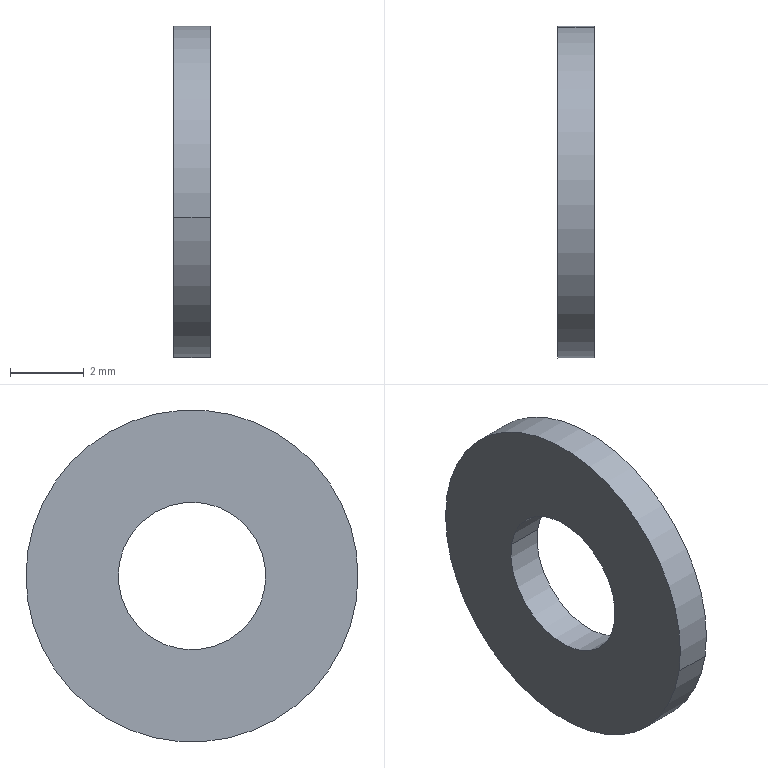Part | SolidWorks | features BaseBody 1 | 1 solid | 6 faces | box 1 x 9 x 9 mm | volume 51.051 mm3 | cylinder 4 | plane 2 | commonest cylinder face diameters 4 x2 9 x2
STEP:
#1=CARTESIAN_POINT('',(-440.148,436.692,-362.691));
#2=VERTEX_POINT('',#1);
#3=CARTESIAN_POINT('',(-440.148,432.739,-363.301));
#4=VERTEX_POINT('',#3);
#5=CARTESIAN_POINT('',(-440.148,434.715,-362.996));
#6=DIRECTION('',(1.,0.,0.));
#7=DIRECTION('',(0.,0.9883,0.1525));
#8=AXIS2_PLACEMENT_3D('',#5,#6,#7);
#9=CIRCLE('',#8,2.);
#10=EDGE_CURVE('',#2,#4,#9,.T.);
#11=ORIENTED_EDGE('',*,*,#10,.F.);
#12=CARTESIAN_POINT('',(-440.148,434.715,-362.996));
#13=DIRECTION('',(1.,0.,0.));
#14=DIRECTION('',(0.,-0.9883,-0.1525));
#15=AXIS2_PLACEMENT_3D('',#12,#13,#14);
#16=CIRCLE('',#15,2.);
#17=EDGE_CURVE('',#4,#2,#16,.T.);
#18=ORIENTED_EDGE('',*,*,#17,.F.);
#19=EDGE_LOOP('',(#11,#18));
#20=FACE_BOUND('',#19,.T.);
#21=CARTESIAN_POINT('',(-440.148,439.163,-362.31));
#22=VERTEX_POINT('',#21);
#23=CARTESIAN_POINT('',(-440.148,430.268,-363.683));
#24=VERTEX_POINT('',#23);
#25=CARTESIAN_POINT('',(-440.148,434.715,-362.996));
#26=DIRECTION('',(-1.,0.,0.));
#27=DIRECTION('',(0.,0.9883,0.1525));
#28=AXIS2_PLACEMENT_3D('',#25,#26,#27);
#29=CIRCLE('',#28,4.5);
#30=EDGE_CURVE('',#22,#24,#29,.T.);
#31=ORIENTED_EDGE('',*,*,#30,.F.);
#32=CARTESIAN_POINT('',(-440.148,434.715,-362.996));
#33=DIRECTION('',(-1.,0.,0.));
#34=DIRECTION('',(0.,-0.9883,-0.1525));
#35=AXIS2_PLACEMENT_3D('',#32,#33,#34);
#36=CIRCLE('',#35,4.5);
#37=EDGE_CURVE('',#24,#22,#36,.T.);
#38=ORIENTED_EDGE('',*,*,#37,.F.);
#39=EDGE_LOOP('',(#31,#38));
#40=FACE_OUTER_BOUND('',#39,.T.);
#41=CARTESIAN_POINT('',(-440.148,434.715,-362.996));
#42=DIRECTION('',(-1.,0.,0.));
#43=DIRECTION('',(0.,0.,1.));
#44=AXIS2_PLACEMENT_3D('',#41,#42,#43);
#45=PLANE('',#44);
#46=ADVANCED_FACE('',(#20,#40),#45,.F.);
#47=CARTESIAN_POINT('',(-441.148,439.163,-362.31));
#48=VERTEX_POINT('',#47);
#49=CARTESIAN_POINT('',(-440.148,439.163,-362.31));
#50=DIRECTION('',(-1.,0.,0.));
#51=VECTOR('',#50,1000.);
#52=LINE('',#49,#51);
#53=EDGE_CURVE('',#22,#48,#52,.T.);
#54=ORIENTED_EDGE('',*,*,#53,.T.);
#55=CARTESIAN_POINT('',(-441.148,430.268,-363.683));
#56=VERTEX_POINT('',#55);
#57=CARTESIAN_POINT('',(-441.148,434.715,-362.996));
#58=DIRECTION('',(1.,0.,0.));
#59=DIRECTION('',(0.,0.9883,0.1525));
#60=AXIS2_PLACEMENT_3D('',#57,#58,#59);
#61=CIRCLE('',#60,4.5);
#62=EDGE_CURVE('',#48,#56,#61,.T.);
#63=ORIENTED_EDGE('',*,*,#62,.T.);
#64=CARTESIAN_POINT('',(-440.148,430.268,-363.683));
#65=DIRECTION('',(-1.,0.,0.));
#66=VECTOR('',#65,1000.);
#67=LINE('',#64,#66);
#68=EDGE_CURVE('',#24,#56,#67,.T.);
#69=ORIENTED_EDGE('',*,*,#68,.F.);
#70=ORIENTED_EDGE('',*,*,#37,.T.);
#71=EDGE_LOOP('',(#54,#63,#69,#70));
#72=FACE_OUTER_BOUND('',#71,.T.);
#73=CARTESIAN_POINT('',(-440.148,434.715,-362.996));
#74=DIRECTION('',(-1.,0.,0.));
#75=DIRECTION('',(0.,-0.9883,-0.1525));
#76=AXIS2_PLACEMENT_3D('',#73,#74,#75);
#77=CYLINDRICAL_SURFACE('',#76,4.5);
#78=ADVANCED_FACE('',(#72),#77,.T.);
#79=ORIENTED_EDGE('',*,*,#68,.T.);
#80=CARTESIAN_POINT('',(-441.148,434.715,-362.996));
#81=DIRECTION('',(1.,0.,0.));
#82=DIRECTION('',(0.,-0.9883,-0.1525));
#83=AXIS2_PLACEMENT_3D('',#80,#81,#82);
#84=CIRCLE('',#83,4.5);
#85=EDGE_CURVE('',#56,#48,#84,.T.);
#86=ORIENTED_EDGE('',*,*,#85,.T.);
#87=ORIENTED_EDGE('',*,*,#53,.F.);
#88=ORIENTED_EDGE('',*,*,#30,.T.);
#89=EDGE_LOOP('',(#79,#86,#87,#88));
#90=FACE_OUTER_BOUND('',#89,.T.);
#91=CARTESIAN_POINT('',(-440.148,434.715,-362.996));
#92=DIRECTION('',(-1.,0.,0.));
#93=DIRECTION('',(0.,-0.9883,-0.1525));
#94=AXIS2_PLACEMENT_3D('',#91,#92,#93);
#95=CYLINDRICAL_SURFACE('',#94,4.5);
#96=ADVANCED_FACE('',(#90),#95,.T.);
#97=CARTESIAN_POINT('',(-441.148,432.739,-363.301));
#98=VERTEX_POINT('',#97);
#99=CARTESIAN_POINT('',(-441.148,436.692,-362.691));
#100=VERTEX_POINT('',#99);
#101=CARTESIAN_POINT('',(-441.148,434.715,-362.996));
#102=DIRECTION('',(-1.,0.,0.));
#103=DIRECTION('',(0.,-0.9883,-0.1525));
#104=AXIS2_PLACEMENT_3D('',#101,#102,#103);
#105=CIRCLE('',#104,2.);
#106=EDGE_CURVE('',#98,#100,#105,.T.);
#107=ORIENTED_EDGE('',*,*,#106,.F.);
#108=CARTESIAN_POINT('',(-441.148,434.715,-362.996));
#109=DIRECTION('',(-1.,0.,0.));
#110=DIRECTION('',(0.,0.9883,0.1525));
#111=AXIS2_PLACEMENT_3D('',#108,#109,#110);
#112=CIRCLE('',#111,2.);
#113=EDGE_CURVE('',#100,#98,#112,.T.);
#114=ORIENTED_EDGE('',*,*,#113,.F.);
#115=EDGE_LOOP('',(#107,#114));
#116=FACE_BOUND('',#115,.T.);
#117=ORIENTED_EDGE('',*,*,#85,.F.);
#118=ORIENTED_EDGE('',*,*,#62,.F.);
#119=EDGE_LOOP('',(#117,#118));
#120=FACE_OUTER_BOUND('',#119,.T.);
#121=CARTESIAN_POINT('',(-441.148,434.715,-362.996));
#122=DIRECTION('',(-1.,0.,0.));
#123=DIRECTION('',(0.,0.,1.));
#124=AXIS2_PLACEMENT_3D('',#121,#122,#123);
#125=PLANE('',#124);
#126=ADVANCED_FACE('',(#116,#120),#125,.T.);
#127=CARTESIAN_POINT('',(-440.148,436.692,-362.691));
#128=DIRECTION('',(-1.,0.,0.));
#129=VECTOR('',#128,1000.);
#130=LINE('',#127,#129);
#131=EDGE_CURVE('',#2,#100,#130,.T.);
#132=ORIENTED_EDGE('',*,*,#131,.T.);
#133=ORIENTED_EDGE('',*,*,#113,.T.);
#134=CARTESIAN_POINT('',(-440.148,432.739,-363.301));
#135=DIRECTION('',(-1.,0.,0.));
#136=VECTOR('',#135,1000.);
#137=LINE('',#134,#136);
#138=EDGE_CURVE('',#4,#98,#137,.T.);
#139=ORIENTED_EDGE('',*,*,#138,.F.);
#140=ORIENTED_EDGE('',*,*,#17,.T.);
#141=EDGE_LOOP('',(#132,#133,#139,#140));
#142=FACE_OUTER_BOUND('',#141,.T.);
#143=CARTESIAN_POINT('',(-440.148,434.715,-362.996));
#144=DIRECTION('',(-1.,0.,0.));
#145=DIRECTION('',(0.,-0.9883,-0.1525));
#146=AXIS2_PLACEMENT_3D('',#143,#144,#145);
#147=CYLINDRICAL_SURFACE('',#146,2.);
#148=ADVANCED_FACE('',(#142),#147,.F.);
#149=ORIENTED_EDGE('',*,*,#138,.T.);
#150=ORIENTED_EDGE('',*,*,#106,.T.);
#151=ORIENTED_EDGE('',*,*,#131,.F.);
#152=ORIENTED_EDGE('',*,*,#10,.T.);
#153=EDGE_LOOP('',(#149,#150,#151,#152));
#154=FACE_OUTER_BOUND('',#153,.T.);
#155=CARTESIAN_POINT('',(-440.148,434.715,-362.996));
#156=DIRECTION('',(-1.,0.,0.));
#157=DIRECTION('',(0.,-0.9883,-0.1525));
#158=AXIS2_PLACEMENT_3D('',#155,#156,#157);
#159=CYLINDRICAL_SURFACE('',#158,2.);
#160=ADVANCED_FACE('',(#154),#159,.F.);
#161=CLOSED_SHELL('',(#46,#78,#96,#126,#148,#160));
#162=MANIFOLD_SOLID_BREP('',#161);
#163=CARTESIAN_POINT('',(0.,0.,0.));
#164=DIRECTION('',(0.,0.,1.));
#165=DIRECTION('',(1.,0.,0.));
#166=AXIS2_PLACEMENT_3D('',#163,#164,#165);
#167=(LENGTH_UNIT()NAMED_UNIT(*)SI_UNIT(.MILLI.,.METRE.));
#168=UNCERTAINTY_MEASURE_WITH_UNIT(LENGTH_MEASURE(0.00001),#167,'','');
#169=(NAMED_UNIT(*)PLANE_ANGLE_UNIT()SI_UNIT($,.RADIAN.));
#170=(NAMED_UNIT(*)SI_UNIT($,.STERADIAN.)SOLID_ANGLE_UNIT());
#171=(GEOMETRIC_REPRESENTATION_CONTEXT(3)GLOBAL_UNCERTAINTY_ASSIGNED_CONTEXT((#168))GLOBAL_UNIT_ASSIGNED_CONTEXT((#167,#169,#170))REPRESENTATION_CONTEXT('',''));
#172=ADVANCED_BREP_SHAPE_REPRESENTATION('',(#162,#166),#171);